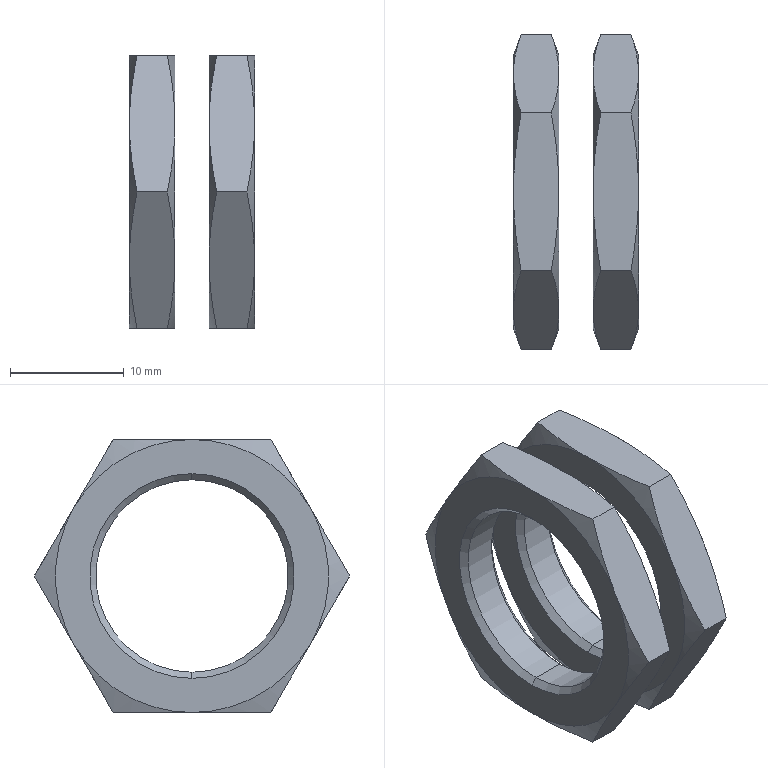Part | SolidWorks | features AEMSimFeature 1 | 2 solids | 52 faces | box 11 x 27.713 x 24 mm | volume 2123 mm3 | cone 32 | plane 16 | cylinder 4 | commonest cylinder face diameters 16.917 x4